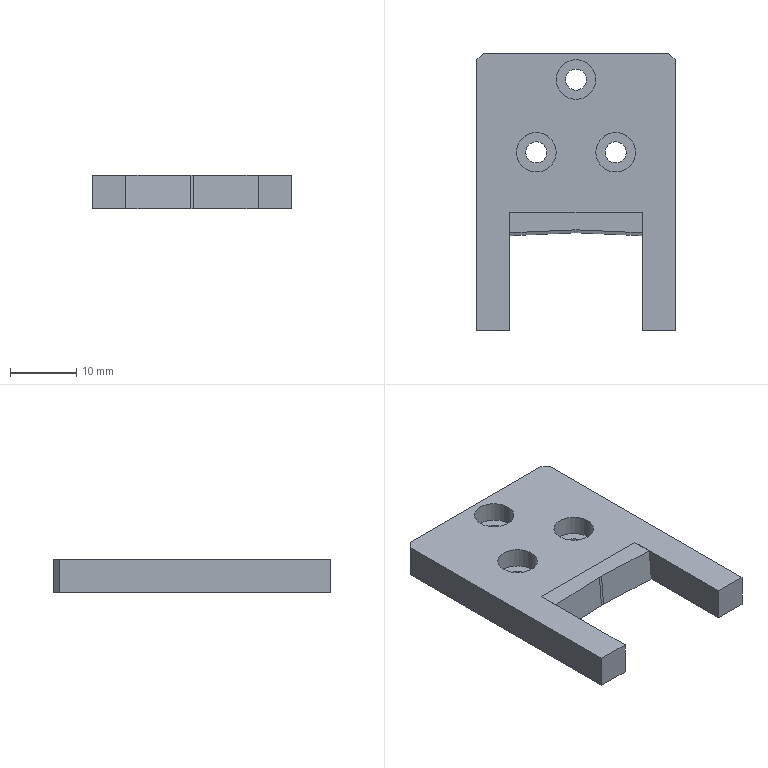Part | SolidWorks | features ICE 3, Chamfer 2, Extrusion 1, Fillet 1, HoleWzd 1 | 2 solids | 35 faces | box 30 x 42 x 5 mm | volume 4509 mm3 | plane 22 | cylinder 13 | commonest cylinder face diameters 3.2 x6 6 x6 10 x1
STEP:
#1=CARTESIAN_POINT('',(-18.,-4.,-0.5));
#2=VERTEX_POINT('',#1);
#3=CARTESIAN_POINT('',(-12.,-4.,-0.5));
#4=VERTEX_POINT('',#3);
#5=CARTESIAN_POINT('',(-15.,-4.,-0.5));
#6=DIRECTION('',(0.,0.,1.));
#7=DIRECTION('',(1.,0.,0.));
#8=AXIS2_PLACEMENT_3D('',#5,#6,#7);
#9=CIRCLE('',#8,3.);
#10=EDGE_CURVE('',#2,#4,#9,.T.);
#11=ORIENTED_EDGE('',*,*,#10,.F.);
#12=CARTESIAN_POINT('',(-18.,-4.,2.5));
#13=VERTEX_POINT('',#12);
#14=CARTESIAN_POINT('',(-18.,-4.,2.5));
#15=DIRECTION('',(0.,0.,1.));
#16=VECTOR('',#15,1000.);
#17=LINE('',#14,#16);
#18=EDGE_CURVE('',#2,#13,#17,.T.);
#19=ORIENTED_EDGE('',*,*,#18,.T.);
#20=CARTESIAN_POINT('',(-12.,-4.,2.5));
#21=VERTEX_POINT('',#20);
#22=CARTESIAN_POINT('',(-15.,-4.,2.5));
#23=DIRECTION('',(0.,0.,1.));
#24=DIRECTION('',(1.,0.,0.));
#25=AXIS2_PLACEMENT_3D('',#22,#23,#24);
#26=CIRCLE('',#25,3.);
#27=EDGE_CURVE('',#13,#21,#26,.T.);
#28=ORIENTED_EDGE('',*,*,#27,.T.);
#29=CARTESIAN_POINT('',(-12.,-4.,2.5));
#30=DIRECTION('',(0.,0.,1.));
#31=VECTOR('',#30,1000.);
#32=LINE('',#29,#31);
#33=EDGE_CURVE('',#4,#21,#32,.T.);
#34=ORIENTED_EDGE('',*,*,#33,.F.);
#35=EDGE_LOOP('',(#11,#19,#28,#34));
#36=FACE_OUTER_BOUND('',#35,.T.);
#37=CARTESIAN_POINT('',(-15.,-4.,2.5));
#38=DIRECTION('',(0.,0.,1.));
#39=DIRECTION('',(1.,0.,0.));
#40=AXIS2_PLACEMENT_3D('',#37,#38,#39);
#41=CYLINDRICAL_SURFACE('',#40,3.);
#42=ADVANCED_FACE('',(#36),#41,.F.);
#43=CARTESIAN_POINT('',(-16.6,-4.,-2.5));
#44=VERTEX_POINT('',#43);
#45=CARTESIAN_POINT('',(-13.4,-4.,-2.5));
#46=VERTEX_POINT('',#45);
#47=CARTESIAN_POINT('',(-15.,-4.,-2.5));
#48=DIRECTION('',(0.,0.,1.));
#49=DIRECTION('',(1.,0.,0.));
#50=AXIS2_PLACEMENT_3D('',#47,#48,#49);
#51=CIRCLE('',#50,1.6);
#52=EDGE_CURVE('',#44,#46,#51,.T.);
#53=ORIENTED_EDGE('',*,*,#52,.F.);
#54=CARTESIAN_POINT('',(-16.6,-4.,-0.5));
#55=VERTEX_POINT('',#54);
#56=CARTESIAN_POINT('',(-16.6,-4.,2.5));
#57=DIRECTION('',(0.,0.,1.));
#58=VECTOR('',#57,1000.);
#59=LINE('',#56,#58);
#60=EDGE_CURVE('',#44,#55,#59,.T.);
#61=ORIENTED_EDGE('',*,*,#60,.T.);
#62=CARTESIAN_POINT('',(-13.4,-4.,-0.5));
#63=VERTEX_POINT('',#62);
#64=CARTESIAN_POINT('',(-15.,-4.,-0.5));
#65=DIRECTION('',(0.,0.,1.));
#66=DIRECTION('',(1.,0.,0.));
#67=AXIS2_PLACEMENT_3D('',#64,#65,#66);
#68=CIRCLE('',#67,1.6);
#69=EDGE_CURVE('',#55,#63,#68,.T.);
#70=ORIENTED_EDGE('',*,*,#69,.T.);
#71=CARTESIAN_POINT('',(-13.4,-4.,2.5));
#72=DIRECTION('',(0.,0.,1.));
#73=VECTOR('',#72,1000.);
#74=LINE('',#71,#73);
#75=EDGE_CURVE('',#46,#63,#74,.T.);
#76=ORIENTED_EDGE('',*,*,#75,.F.);
#77=EDGE_LOOP('',(#53,#61,#70,#76));
#78=FACE_OUTER_BOUND('',#77,.T.);
#79=CARTESIAN_POINT('',(-15.,-4.,2.5));
#80=DIRECTION('',(0.,0.,1.));
#81=DIRECTION('',(1.,0.,0.));
#82=AXIS2_PLACEMENT_3D('',#79,#80,#81);
#83=CYLINDRICAL_SURFACE('',#82,1.6);
#84=ADVANCED_FACE('',(#78),#83,.F.);
#85=CARTESIAN_POINT('',(-24.,-15.,-0.5));
#86=VERTEX_POINT('',#85);
#87=CARTESIAN_POINT('',(-18.,-15.,-0.5));
#88=VERTEX_POINT('',#87);
#89=CARTESIAN_POINT('',(-21.,-15.,-0.5));
#90=DIRECTION('',(0.,0.,1.));
#91=DIRECTION('',(1.,0.,0.));
#92=AXIS2_PLACEMENT_3D('',#89,#90,#91);
#93=CIRCLE('',#92,3.);
#94=EDGE_CURVE('',#86,#88,#93,.T.);
#95=ORIENTED_EDGE('',*,*,#94,.F.);
#96=CARTESIAN_POINT('',(-24.,-15.,2.5));
#97=VERTEX_POINT('',#96);
#98=CARTESIAN_POINT('',(-24.,-15.,2.5));
#99=DIRECTION('',(0.,0.,1.));
#100=VECTOR('',#99,1000.);
#101=LINE('',#98,#100);
#102=EDGE_CURVE('',#86,#97,#101,.T.);
#103=ORIENTED_EDGE('',*,*,#102,.T.);
#104=CARTESIAN_POINT('',(-18.,-15.,2.5));
#105=VERTEX_POINT('',#104);
#106=CARTESIAN_POINT('',(-21.,-15.,2.5));
#107=DIRECTION('',(0.,0.,1.));
#108=DIRECTION('',(1.,0.,0.));
#109=AXIS2_PLACEMENT_3D('',#106,#107,#108);
#110=CIRCLE('',#109,3.);
#111=EDGE_CURVE('',#97,#105,#110,.T.);
#112=ORIENTED_EDGE('',*,*,#111,.T.);
#113=CARTESIAN_POINT('',(-18.,-15.,2.5));
#114=DIRECTION('',(0.,0.,1.));
#115=VECTOR('',#114,1000.);
#116=LINE('',#113,#115);
#117=EDGE_CURVE('',#88,#105,#116,.T.);
#118=ORIENTED_EDGE('',*,*,#117,.F.);
#119=EDGE_LOOP('',(#95,#103,#112,#118));
#120=FACE_OUTER_BOUND('',#119,.T.);
#121=CARTESIAN_POINT('',(-21.,-15.,2.5));
#122=DIRECTION('',(0.,0.,1.));
#123=DIRECTION('',(1.,0.,0.));
#124=AXIS2_PLACEMENT_3D('',#121,#122,#123);
#125=CYLINDRICAL_SURFACE('',#124,3.);
#126=ADVANCED_FACE('',(#120),#125,.F.);
#127=CARTESIAN_POINT('',(-22.6,-15.,-2.5));
#128=VERTEX_POINT('',#127);
#129=CARTESIAN_POINT('',(-19.4,-15.,-2.5));
#130=VERTEX_POINT('',#129);
#131=CARTESIAN_POINT('',(-21.,-15.,-2.5));
#132=DIRECTION('',(0.,0.,1.));
#133=DIRECTION('',(1.,0.,0.));
#134=AXIS2_PLACEMENT_3D('',#131,#132,#133);
#135=CIRCLE('',#134,1.6);
#136=EDGE_CURVE('',#128,#130,#135,.T.);
#137=ORIENTED_EDGE('',*,*,#136,.F.);
#138=CARTESIAN_POINT('',(-22.6,-15.,-0.5));
#139=VERTEX_POINT('',#138);
#140=CARTESIAN_POINT('',(-22.6,-15.,2.5));
#141=DIRECTION('',(0.,0.,1.));
#142=VECTOR('',#141,1000.);
#143=LINE('',#140,#142);
#144=EDGE_CURVE('',#128,#139,#143,.T.);
#145=ORIENTED_EDGE('',*,*,#144,.T.);
#146=CARTESIAN_POINT('',(-19.4,-15.,-0.5));
#147=VERTEX_POINT('',#146);
#148=CARTESIAN_POINT('',(-21.,-15.,-0.5));
#149=DIRECTION('',(0.,0.,1.));
#150=DIRECTION('',(1.,0.,0.));
#151=AXIS2_PLACEMENT_3D('',#148,#149,#150);
#152=CIRCLE('',#151,1.6);
#153=EDGE_CURVE('',#139,#147,#152,.T.);
#154=ORIENTED_EDGE('',*,*,#153,.T.);
#155=CARTESIAN_POINT('',(-19.4,-15.,2.5));
#156=DIRECTION('',(0.,0.,1.));
#157=VECTOR('',#156,1000.);
#158=LINE('',#155,#157);
#159=EDGE_CURVE('',#130,#147,#158,.T.);
#160=ORIENTED_EDGE('',*,*,#159,.F.);
#161=EDGE_LOOP('',(#137,#145,#154,#160));
#162=FACE_OUTER_BOUND('',#161,.T.);
#163=CARTESIAN_POINT('',(-21.,-15.,2.5));
#164=DIRECTION('',(0.,0.,1.));
#165=DIRECTION('',(1.,0.,0.));
#166=AXIS2_PLACEMENT_3D('',#163,#164,#165);
#167=CYLINDRICAL_SURFACE('',#166,1.6);
#168=ADVANCED_FACE('',(#162),#167,.F.);
#169=CARTESIAN_POINT('',(-12.,-15.,-0.5));
#170=VERTEX_POINT('',#169);
#171=CARTESIAN_POINT('',(-6.,-15.,-0.5));
#172=VERTEX_POINT('',#171);
#173=CARTESIAN_POINT('',(-9.,-15.,-0.5));
#174=DIRECTION('',(0.,0.,1.));
#175=DIRECTION('',(1.,0.,0.));
#176=AXIS2_PLACEMENT_3D('',#173,#174,#175);
#177=CIRCLE('',#176,3.);
#178=EDGE_CURVE('',#170,#172,#177,.T.);
#179=ORIENTED_EDGE('',*,*,#178,.F.);
#180=CARTESIAN_POINT('',(-12.,-15.,2.5));
#181=VERTEX_POINT('',#180);
#182=CARTESIAN_POINT('',(-12.,-15.,2.5));
#183=DIRECTION('',(0.,0.,1.));
#184=VECTOR('',#183,1000.);
#185=LINE('',#182,#184);
#186=EDGE_CURVE('',#170,#181,#185,.T.);
#187=ORIENTED_EDGE('',*,*,#186,.T.);
#188=CARTESIAN_POINT('',(-6.,-15.,2.5));
#189=VERTEX_POINT('',#188);
#190=CARTESIAN_POINT('',(-9.,-15.,2.5));
#191=DIRECTION('',(0.,0.,1.));
#192=DIRECTION('',(1.,0.,0.));
#193=AXIS2_PLACEMENT_3D('',#190,#191,#192);
#194=CIRCLE('',#193,3.);
#195=EDGE_CURVE('',#181,#189,#194,.T.);
#196=ORIENTED_EDGE('',*,*,#195,.T.);
#197=CARTESIAN_POINT('',(-6.,-15.,2.5));
#198=DIRECTION('',(0.,0.,1.));
#199=VECTOR('',#198,1000.);
#200=LINE('',#197,#199);
#201=EDGE_CURVE('',#172,#189,#200,.T.);
#202=ORIENTED_EDGE('',*,*,#201,.F.);
#203=EDGE_LOOP('',(#179,#187,#196,#202));
#204=FACE_OUTER_BOUND('',#203,.T.);
#205=CARTESIAN_POINT('',(-9.,-15.,2.5));
#206=DIRECTION('',(0.,0.,1.));
#207=DIRECTION('',(1.,0.,0.));
#208=AXIS2_PLACEMENT_3D('',#205,#206,#207);
#209=CYLINDRICAL_SURFACE('',#208,3.);
#210=ADVANCED_FACE('',(#204),#209,.F.);
#211=CARTESIAN_POINT('',(-10.6,-15.,-2.5));
#212=VERTEX_POINT('',#211);
#213=CARTESIAN_POINT('',(-7.4,-15.,-2.5));
#214=VERTEX_POINT('',#213);
#215=CARTESIAN_POINT('',(-9.,-15.,-2.5));
#216=DIRECTION('',(0.,0.,1.));
#217=DIRECTION('',(1.,0.,0.));
#218=AXIS2_PLACEMENT_3D('',#215,#216,#217);
#219=CIRCLE('',#218,1.6);
#220=EDGE_CURVE('',#212,#214,#219,.T.);
#221=ORIENTED_EDGE('',*,*,#220,.F.);
#222=CARTESIAN_POINT('',(-10.6,-15.,-0.5));
#223=VERTEX_POINT('',#222);
#224=CARTESIAN_POINT('',(-10.6,-15.,2.5));
#225=DIRECTION('',(0.,0.,1.));
#226=VECTOR('',#225,1000.);
#227=LINE('',#224,#226);
#228=EDGE_CURVE('',#212,#223,#227,.T.);
#229=ORIENTED_EDGE('',*,*,#228,.T.);
#230=CARTESIAN_POINT('',(-7.4,-15.,-0.5));
#231=VERTEX_POINT('',#230);
#232=CARTESIAN_POINT('',(-9.,-15.,-0.5));
#233=DIRECTION('',(0.,0.,1.));
#234=DIRECTION('',(1.,0.,0.));
#235=AXIS2_PLACEMENT_3D('',#232,#233,#234);
#236=CIRCLE('',#235,1.6);
#237=EDGE_CURVE('',#223,#231,#236,.T.);
#238=ORIENTED_EDGE('',*,*,#237,.T.);
#239=CARTESIAN_POINT('',(-7.4,-15.,2.5));
#240=DIRECTION('',(0.,0.,1.));
#241=VECTOR('',#240,1000.);
#242=LINE('',#239,#241);
#243=EDGE_CURVE('',#214,#231,#242,.T.);
#244=ORIENTED_EDGE('',*,*,#243,.F.);
#245=EDGE_LOOP('',(#221,#229,#238,#244));
#246=FACE_OUTER_BOUND('',#245,.T.);
#247=CARTESIAN_POINT('',(-9.,-15.,2.5));
#248=DIRECTION('',(0.,0.,1.));
#249=DIRECTION('',(1.,0.,0.));
#250=AXIS2_PLACEMENT_3D('',#247,#248,#249);
#251=CYLINDRICAL_SURFACE('',#250,1.6);
#252=ADVANCED_FACE('',(#246),#251,.F.);
#253=CARTESIAN_POINT('',(0.,-42.,-2.5));
#254=VERTEX_POINT('',#253);
#255=CARTESIAN_POINT('',(0.,-1.,-2.5));
#256=VERTEX_POINT('',#255);
#257=CARTESIAN_POINT('',(0.,0.,-2.5));
#258=DIRECTION('',(0.,1.,0.));
#259=VECTOR('',#258,1000.);
#260=LINE('',#257,#259);
#261=EDGE_CURVE('',#254,#256,#260,.T.);
#262=ORIENTED_EDGE('',*,*,#261,.T.);
#263=CARTESIAN_POINT('',(0.,-1.,2.5));
#264=VERTEX_POINT('',#263);
#265=CARTESIAN_POINT('',(0.,-1.,2.5));
#266=DIRECTION('',(0.,0.,1.));
#267=VECTOR('',#266,1000.);
#268=LINE('',#265,#267);
#269=EDGE_CURVE('',#256,#264,#268,.T.);
#270=ORIENTED_EDGE('',*,*,#269,.T.);
#271=CARTESIAN_POINT('',(0.,-42.,2.5));
#272=VERTEX_POINT('',#271);
#273=CARTESIAN_POINT('',(0.,0.,2.5));
#274=DIRECTION('',(0.,1.,0.));
#275=VECTOR('',#274,1000.);
#276=LINE('',#273,#275);
#277=EDGE_CURVE('',#272,#264,#276,.T.);
#278=ORIENTED_EDGE('',*,*,#277,.F.);
#279=CARTESIAN_POINT('',(0.,-42.,2.5));
#280=DIRECTION('',(0.,0.,-1.));
#281=VECTOR('',#280,1000.);
#282=LINE('',#279,#281);
#283=EDGE_CURVE('',#272,#254,#282,.T.);
#284=ORIENTED_EDGE('',*,*,#283,.T.);
#285=EDGE_LOOP('',(#262,#270,#278,#284));
#286=FACE_OUTER_BOUND('',#285,.T.);
#287=CARTESIAN_POINT('',(0.,0.,2.5));
#288=DIRECTION('',(-1.,0.,0.));
#289=DIRECTION('',(0.,-1.,0.));
#290=AXIS2_PLACEMENT_3D('',#287,#288,#289);
#291=PLANE('',#290);
#292=ADVANCED_FACE('',(#286),#291,.F.);
#293=CARTESIAN_POINT('',(-1.,0.,2.5));
#294=VERTEX_POINT('',#293);
#295=CARTESIAN_POINT('',(-29.,0.,2.5));
#296=VERTEX_POINT('',#295);
#297=CARTESIAN_POINT('',(0.,0.,2.5));
#298=DIRECTION('',(-1.,0.,0.));
#299=VECTOR('',#298,1000.);
#300=LINE('',#297,#299);
#301=EDGE_CURVE('',#294,#296,#300,.T.);
#302=ORIENTED_EDGE('',*,*,#301,.F.);
#303=CARTESIAN_POINT('',(-1.,0.,-2.5));
#304=VERTEX_POINT('',#303);
#305=CARTESIAN_POINT('',(-1.,0.,2.5));
#306=DIRECTION('',(0.,0.,-1.));
#307=VECTOR('',#306,1000.);
#308=LINE('',#305,#307);
#309=EDGE_CURVE('',#294,#304,#308,.T.);
#310=ORIENTED_EDGE('',*,*,#309,.T.);
#311=CARTESIAN_POINT('',(-29.,0.,-2.5));
#312=VERTEX_POINT('',#311);
#313=CARTESIAN_POINT('',(0.,0.,-2.5));
#314=DIRECTION('',(-1.,0.,0.));
#315=VECTOR('',#314,1000.);
#316=LINE('',#313,#315);
#317=EDGE_CURVE('',#304,#312,#316,.T.);
#318=ORIENTED_EDGE('',*,*,#317,.T.);
#319=CARTESIAN_POINT('',(-29.,0.,2.5));
#320=DIRECTION('',(0.,0.,1.));
#321=VECTOR('',#320,1000.);
#322=LINE('',#319,#321);
#323=EDGE_CURVE('',#312,#296,#322,.T.);
#324=ORIENTED_EDGE('',*,*,#323,.T.);
#325=EDGE_LOOP('',(#302,#310,#318,#324));
#326=FACE_OUTER_BOUND('',#325,.T.);
#327=CARTESIAN_POINT('',(0.,0.,2.5));
#328=DIRECTION('',(0.,-1.,0.));
#329=DIRECTION('',(1.,0.,0.));
#330=AXIS2_PLACEMENT_3D('',#327,#328,#329);
#331=PLANE('',#330);
#332=ADVANCED_FACE('',(#326),#331,.F.);
#333=CARTESIAN_POINT('',(-30.,-1.,2.5));
#334=VERTEX_POINT('',#333);
#335=CARTESIAN_POINT('',(-30.,-42.,2.5));
#336=VERTEX_POINT('',#335);
#337=CARTESIAN_POINT('',(-30.,0.,2.5));
#338=DIRECTION('',(0.,-1.,0.));
#339=VECTOR('',#338,1000.);
#340=LINE('',#337,#339);
#341=EDGE_CURVE('',#334,#336,#340,.T.);
#342=ORIENTED_EDGE('',*,*,#341,.F.);
#343=CARTESIAN_POINT('',(-30.,-1.,-2.5));
#344=VERTEX_POINT('',#343);
#345=CARTESIAN_POINT('',(-30.,-1.,2.5));
#346=DIRECTION('',(0.,0.,-1.));
#347=VECTOR('',#346,1000.);
#348=LINE('',#345,#347);
#349=EDGE_CURVE('',#334,#344,#348,.T.);
#350=ORIENTED_EDGE('',*,*,#349,.T.);
#351=CARTESIAN_POINT('',(-30.,-42.,-2.5));
#352=VERTEX_POINT('',#351);
#353=CARTESIAN_POINT('',(-30.,0.,-2.5));
#354=DIRECTION('',(0.,-1.,0.));
#355=VECTOR('',#354,1000.);
#356=LINE('',#353,#355);
#357=EDGE_CURVE('',#344,#352,#356,.T.);
#358=ORIENTED_EDGE('',*,*,#357,.T.);
#359=CARTESIAN_POINT('',(-30.,-42.,2.5));
#360=DIRECTION('',(0.,0.,-1.));
#361=VECTOR('',#360,1000.);
#362=LINE('',#359,#361);
#363=EDGE_CURVE('',#336,#352,#362,.T.);
#364=ORIENTED_EDGE('',*,*,#363,.F.);
#365=EDGE_LOOP('',(#342,#350,#358,#364));
#366=FACE_OUTER_BOUND('',#365,.T.);
#367=CARTESIAN_POINT('',(-30.,0.,2.5));
#368=DIRECTION('',(1.,0.,0.));
#369=DIRECTION('',(0.,1.,0.));
#370=AXIS2_PLACEMENT_3D('',#367,#368,#369);
#371=PLANE('',#370);
#372=ADVANCED_FACE('',(#366),#371,.F.);
#373=CARTESIAN_POINT('',(-25.,-42.,-2.5));
#374=VERTEX_POINT('',#373);
#375=CARTESIAN_POINT('',(-25.,-42.,-2.5));
#376=DIRECTION('',(1.,0.,0.));
#377=VECTOR('',#376,1000.);
#378=LINE('',#375,#377);
#379=EDGE_CURVE('',#352,#374,#378,.T.);
#380=ORIENTED_EDGE('',*,*,#379,.T.);
#381=CARTESIAN_POINT('',(-25.,-42.,2.5));
#382=VERTEX_POINT('',#381);
#383=CARTESIAN_POINT('',(-25.,-42.,2.5));
#384=DIRECTION('',(0.,0.,-1.));
#385=VECTOR('',#384,1000.);
#386=LINE('',#383,#385);
#387=EDGE_CURVE('',#382,#374,#386,.T.);
#388=ORIENTED_EDGE('',*,*,#387,.F.);
#389=CARTESIAN_POINT('',(-25.,-42.,2.5));
#390=DIRECTION('',(1.,0.,0.));
#391=VECTOR('',#390,1000.);
#392=LINE('',#389,#391);
#393=EDGE_CURVE('',#336,#382,#392,.T.);
#394=ORIENTED_EDGE('',*,*,#393,.F.);
#395=ORIENTED_EDGE('',*,*,#363,.T.);
#396=EDGE_LOOP('',(#380,#388,#394,#395));
#397=FACE_OUTER_BOUND('',#396,.T.);
#398=CARTESIAN_POINT('',(-25.,-42.,2.5));
#399=DIRECTION('',(0.,1.,0.));
#400=DIRECTION('',(-1.,0.,0.));
#401=AXIS2_PLACEMENT_3D('',#398,#399,#400);
#402=PLANE('',#401);
#403=ADVANCED_FACE('',(#397),#402,.F.);
#404=CARTESIAN_POINT('',(-25.,-24.1,-2.5));
#405=VERTEX_POINT('',#404);
#406=CARTESIAN_POINT('',(-25.,-24.1,-2.5));
#407=DIRECTION('',(0.,1.,0.));
#408=VECTOR('',#407,1000.);
#409=LINE('',#406,#408);
#410=EDGE_CURVE('',#374,#405,#409,.T.);
#411=ORIENTED_EDGE('',*,*,#410,.T.);
#412=CARTESIAN_POINT('',(-25.,-24.1,2.5));
#413=VERTEX_POINT('',#412);
#414=CARTESIAN_POINT('',(-25.,-24.1,2.5));
#415=DIRECTION('',(0.,0.,-1.));
#416=VECTOR('',#415,1000.);
#417=LINE('',#414,#416);
#418=EDGE_CURVE('',#413,#405,#417,.T.);
#419=ORIENTED_EDGE('',*,*,#418,.F.);
#420=CARTESIAN_POINT('',(-25.,-24.1,2.5));
#421=DIRECTION('',(0.,1.,0.));
#422=VECTOR('',#421,1000.);
#423=LINE('',#420,#422);
#424=EDGE_CURVE('',#382,#413,#423,.T.);
#425=ORIENTED_EDGE('',*,*,#424,.F.);
#426=ORIENTED_EDGE('',*,*,#387,.T.);
#427=EDGE_LOOP('',(#411,#419,#425,#426));
#428=FACE_OUTER_BOUND('',#427,.T.);
#429=CARTESIAN_POINT('',(-25.,-24.1,2.5));
#430=DIRECTION('',(-1.,0.,0.));
#431=DIRECTION('',(0.,0.,1.));
#432=AXIS2_PLACEMENT_3D('',#429,#430,#431);
#433=PLANE('',#432);
#434=ADVANCED_FACE('',(#428),#433,.F.);
#435=CARTESIAN_POINT('',(-5.,-24.1,-2.5));
#436=VERTEX_POINT('',#435);
#437=CARTESIAN_POINT('',(-25.,-24.1,-2.5));
#438=DIRECTION('',(1.,0.,0.));
#439=VECTOR('',#438,1000.);
#440=LINE('',#437,#439);
#441=EDGE_CURVE('',#405,#436,#440,.T.);
#442=ORIENTED_EDGE('',*,*,#441,.T.);
#443=CARTESIAN_POINT('',(-5.,-24.1,2.5));
#444=VERTEX_POINT('',#443);
#445=CARTESIAN_POINT('',(-5.,-24.1,2.5));
#446=DIRECTION('',(0.,0.,-1.));
#447=VECTOR('',#446,1000.);
#448=LINE('',#445,#447);
#449=EDGE_CURVE('',#444,#436,#448,.T.);
#450=ORIENTED_EDGE('',*,*,#449,.F.);
#451=CARTESIAN_POINT('',(-25.,-24.1,2.5));
#452=DIRECTION('',(1.,0.,0.));
#453=VECTOR('',#452,1000.);
#454=LINE('',#451,#453);
#455=EDGE_CURVE('',#413,#444,#454,.T.);
#456=ORIENTED_EDGE('',*,*,#455,.F.);
#457=ORIENTED_EDGE('',*,*,#418,.T.);
#458=EDGE_LOOP('',(#442,#450,#456,#457));
#459=FACE_OUTER_BOUND('',#458,.T.);
#460=CARTESIAN_POINT('',(-25.,-24.1,2.5));
#461=DIRECTION('',(0.,1.,0.));
#462=DIRECTION('',(0.,0.,1.));
#463=AXIS2_PLACEMENT_3D('',#460,#461,#462);
#464=PLANE('',#463);
#465=ADVANCED_FACE('',(#459),#464,.F.);
#466=CARTESIAN_POINT('',(-5.,-42.,-2.5));
#467=VERTEX_POINT('',#466);
#468=CARTESIAN_POINT('',(-5.,-42.,-2.5));
#469=DIRECTION('',(0.,-1.,0.));
#470=VECTOR('',#469,1000.);
#471=LINE('',#468,#470);
#472=EDGE_CURVE('',#436,#467,#471,.T.);
#473=ORIENTED_EDGE('',*,*,#472,.T.);
#474=CARTESIAN_POINT('',(-5.,-42.,2.5));
#475=VERTEX_POINT('',#474);
#476=CARTESIAN_POINT('',(-5.,-42.,2.5));
#477=DIRECTION('',(0.,0.,-1.));
#478=VECTOR('',#477,1000.);
#479=LINE('',#476,#478);
#480=EDGE_CURVE('',#475,#467,#479,.T.);
#481=ORIENTED_EDGE('',*,*,#480,.F.);
#482=CARTESIAN_POINT('',(-5.,-42.,2.5));
#483=DIRECTION('',(0.,-1.,0.));
#484=VECTOR('',#483,1000.);
#485=LINE('',#482,#484);
#486=EDGE_CURVE('',#444,#475,#485,.T.);
#487=ORIENTED_EDGE('',*,*,#486,.F.);
#488=ORIENTED_EDGE('',*,*,#449,.T.);
#489=EDGE_LOOP('',(#473,#481,#487,#488));
#490=FACE_OUTER_BOUND('',#489,.T.);
#491=CARTESIAN_POINT('',(-5.,-42.,2.5));
#492=DIRECTION('',(1.,0.,0.));
#493=DIRECTION('',(0.,1.,0.));
#494=AXIS2_PLACEMENT_3D('',#491,#492,#493);
#495=PLANE('',#494);
#496=ADVANCED_FACE('',(#490),#495,.F.);
#497=CARTESIAN_POINT('',(0.,-42.,-2.5));
#498=DIRECTION('',(1.,0.,0.));
#499=VECTOR('',#498,1000.);
#500=LINE('',#497,#499);
#501=EDGE_CURVE('',#467,#254,#500,.T.);
#502=ORIENTED_EDGE('',*,*,#501,.T.);
#503=ORIENTED_EDGE('',*,*,#283,.F.);
#504=CARTESIAN_POINT('',(0.,-42.,2.5));
#505=DIRECTION('',(1.,0.,0.));
#506=VECTOR('',#505,1000.);
#507=LINE('',#504,#506);
#508=EDGE_CURVE('',#475,#272,#507,.T.);
#509=ORIENTED_EDGE('',*,*,#508,.F.);
#510=ORIENTED_EDGE('',*,*,#480,.T.);
#511=EDGE_LOOP('',(#502,#503,#509,#510));
#512=FACE_OUTER_BOUND('',#511,.T.);
#513=CARTESIAN_POINT('',(0.,-42.,2.5));
#514=DIRECTION('',(0.,1.,0.));
#515=DIRECTION('',(0.,0.,1.));
#516=AXIS2_PLACEMENT_3D('',#513,#514,#515);
#517=PLANE('',#516);
#518=ADVANCED_FACE('',(#512),#517,.F.);
#519=CARTESIAN_POINT('',(-15.,-4.,2.5));
#520=DIRECTION('',(0.,0.,1.));
#521=DIRECTION('',(1.,0.,0.));
#522=AXIS2_PLACEMENT_3D('',#519,#520,#521);
#523=CIRCLE('',#522,3.);
#524=EDGE_CURVE('',#21,#13,#523,.T.);
#525=ORIENTED_EDGE('',*,*,#524,.F.);
#526=ORIENTED_EDGE('',*,*,#27,.F.);
#527=EDGE_LOOP('',(#525,#526));
#528=FACE_BOUND('',#527,.T.);
#529=CARTESIAN_POINT('',(-21.,-15.,2.5));
#530=DIRECTION('',(0.,0.,1.));
#531=DIRECTION('',(1.,0.,0.));
#532=AXIS2_PLACEMENT_3D('',#529,#530,#531);
#533=CIRCLE('',#532,3.);
#534=EDGE_CURVE('',#105,#97,#533,.T.);
#535=ORIENTED_EDGE('',*,*,#534,.F.);
#536=ORIENTED_EDGE('',*,*,#111,.F.);
#537=EDGE_LOOP('',(#535,#536));
#538=FACE_BOUND('',#537,.T.);
#539=CARTESIAN_POINT('',(-9.,-15.,2.5));
#540=DIRECTION('',(0.,0.,1.));
#541=DIRECTION('',(1.,0.,0.));
#542=AXIS2_PLACEMENT_3D('',#539,#540,#541);
#543=CIRCLE('',#542,3.);
#544=EDGE_CURVE('',#189,#181,#543,.T.);
#545=ORIENTED_EDGE('',*,*,#544,.F.);
#546=ORIENTED_EDGE('',*,*,#195,.F.);
#547=EDGE_LOOP('',(#545,#546));
#548=FACE_BOUND('',#547,.T.);
#549=ORIENTED_EDGE('',*,*,#277,.T.);
#550=CARTESIAN_POINT('',(-1.,0.,2.5));
#551=DIRECTION('',(-0.7071,0.7071,0.));
#552=VECTOR('',#551,1000.);
#553=LINE('',#550,#552);
#554=EDGE_CURVE('',#264,#294,#553,.T.);
#555=ORIENTED_EDGE('',*,*,#554,.T.);
#556=ORIENTED_EDGE('',*,*,#301,.T.);
#557=CARTESIAN_POINT('',(-30.,-1.,2.5));
#558=DIRECTION('',(-0.7071,-0.7071,0.));
#559=VECTOR('',#558,1000.);
#560=LINE('',#557,#559);
#561=EDGE_CURVE('',#296,#334,#560,.T.);
#562=ORIENTED_EDGE('',*,*,#561,.T.);
#563=ORIENTED_EDGE('',*,*,#341,.T.);
#564=ORIENTED_EDGE('',*,*,#393,.T.);
#565=ORIENTED_EDGE('',*,*,#424,.T.);
#566=ORIENTED_EDGE('',*,*,#455,.T.);
#567=ORIENTED_EDGE('',*,*,#486,.T.);
#568=ORIENTED_EDGE('',*,*,#508,.T.);
#569=EDGE_LOOP('',(#549,#555,#556,#562,#563,#564,#565,#566,#567,#568));
#570=FACE_OUTER_BOUND('',#569,.T.);
#571=CARTESIAN_POINT('',(0.,-42.,2.5));
#572=DIRECTION('',(0.,0.,-1.));
#573=DIRECTION('',(-1.,0.,0.));
#574=AXIS2_PLACEMENT_3D('',#571,#572,#573);
#575=PLANE('',#574);
#576=ADVANCED_FACE('',(#528,#538,#548,#570),#575,.F.);
#577=CARTESIAN_POINT('',(-15.,-4.,-2.5));
#578=DIRECTION('',(0.,0.,1.));
#579=DIRECTION('',(1.,0.,0.));
#580=AXIS2_PLACEMENT_3D('',#577,#578,#579);
#581=CIRCLE('',#580,1.6);
#582=EDGE_CURVE('',#46,#44,#581,.T.);
#583=ORIENTED_EDGE('',*,*,#582,.T.);
#584=ORIENTED_EDGE('',*,*,#52,.T.);
#585=EDGE_LOOP('',(#583,#584));
#586=FACE_BOUND('',#585,.T.);
#587=CARTESIAN_POINT('',(-21.,-15.,-2.5));
#588=DIRECTION('',(0.,0.,1.));
#589=DIRECTION('',(1.,0.,0.));
#590=AXIS2_PLACEMENT_3D('',#587,#588,#589);
#591=CIRCLE('',#590,1.6);
#592=EDGE_CURVE('',#130,#128,#591,.T.);
#593=ORIENTED_EDGE('',*,*,#592,.T.);
#594=ORIENTED_EDGE('',*,*,#136,.T.);
#595=EDGE_LOOP('',(#593,#594));
#596=FACE_BOUND('',#595,.T.);
#597=CARTESIAN_POINT('',(-9.,-15.,-2.5));
#598=DIRECTION('',(0.,0.,1.));
#599=DIRECTION('',(1.,0.,0.));
#600=AXIS2_PLACEMENT_3D('',#597,#598,#599);
#601=CIRCLE('',#600,1.6);
#602=EDGE_CURVE('',#214,#212,#601,.T.);
#603=ORIENTED_EDGE('',*,*,#602,.T.);
#604=ORIENTED_EDGE('',*,*,#220,.T.);
#605=EDGE_LOOP('',(#603,#604));
#606=FACE_BOUND('',#605,.T.);
#607=ORIENTED_EDGE('',*,*,#317,.F.);
#608=CARTESIAN_POINT('',(20.5,-21.5,-2.5));
#609=DIRECTION('',(0.7071,-0.7071,0.));
#610=VECTOR('',#609,1000.);
#611=LINE('',#608,#610);
#612=EDGE_CURVE('',#304,#256,#611,.T.);
#613=ORIENTED_EDGE('',*,*,#612,.T.);
#614=ORIENTED_EDGE('',*,*,#261,.F.);
#615=ORIENTED_EDGE('',*,*,#501,.F.);
#616=ORIENTED_EDGE('',*,*,#472,.F.);
#617=ORIENTED_EDGE('',*,*,#441,.F.);
#618=ORIENTED_EDGE('',*,*,#410,.F.);
#619=ORIENTED_EDGE('',*,*,#379,.F.);
#620=ORIENTED_EDGE('',*,*,#357,.F.);
#621=CARTESIAN_POINT('',(-35.5,-6.5,-2.5));
#622=DIRECTION('',(0.7071,0.7071,0.));
#623=VECTOR('',#622,1000.);
#624=LINE('',#621,#623);
#625=EDGE_CURVE('',#344,#312,#624,.T.);
#626=ORIENTED_EDGE('',*,*,#625,.T.);
#627=EDGE_LOOP('',(#607,#613,#614,#615,#616,#617,#618,#619,#620,#626));
#628=FACE_OUTER_BOUND('',#627,.T.);
#629=CARTESIAN_POINT('',(0.,-42.,-2.5));
#630=DIRECTION('',(0.,0.,-1.));
#631=DIRECTION('',(-1.,0.,0.));
#632=AXIS2_PLACEMENT_3D('',#629,#630,#631);
#633=PLANE('',#632);
#634=ADVANCED_FACE('',(#586,#596,#606,#628),#633,.T.);
#635=ORIENTED_EDGE('',*,*,#228,.F.);
#636=ORIENTED_EDGE('',*,*,#602,.F.);
#637=ORIENTED_EDGE('',*,*,#243,.T.);
#638=CARTESIAN_POINT('',(-9.,-15.,-0.5));
#639=DIRECTION('',(0.,0.,1.));
#640=DIRECTION('',(1.,0.,0.));
#641=AXIS2_PLACEMENT_3D('',#638,#639,#640);
#642=CIRCLE('',#641,1.6);
#643=EDGE_CURVE('',#231,#223,#642,.T.);
#644=ORIENTED_EDGE('',*,*,#643,.T.);
#645=EDGE_LOOP('',(#635,#636,#637,#644));
#646=FACE_OUTER_BOUND('',#645,.T.);
#647=CARTESIAN_POINT('',(-9.,-15.,2.5));
#648=DIRECTION('',(0.,0.,1.));
#649=DIRECTION('',(1.,0.,0.));
#650=AXIS2_PLACEMENT_3D('',#647,#648,#649);
#651=CYLINDRICAL_SURFACE('',#650,1.6);
#652=ADVANCED_FACE('',(#646),#651,.F.);
#653=ORIENTED_EDGE('',*,*,#643,.F.);
#654=ORIENTED_EDGE('',*,*,#237,.F.);
#655=EDGE_LOOP('',(#653,#654));
#656=FACE_BOUND('',#655,.T.);
#657=CARTESIAN_POINT('',(-9.,-15.,-0.5));
#658=DIRECTION('',(0.,0.,1.));
#659=DIRECTION('',(1.,0.,0.));
#660=AXIS2_PLACEMENT_3D('',#657,#658,#659);
#661=CIRCLE('',#660,3.);
#662=EDGE_CURVE('',#172,#170,#661,.T.);
#663=ORIENTED_EDGE('',*,*,#662,.T.);
#664=ORIENTED_EDGE('',*,*,#178,.T.);
#665=EDGE_LOOP('',(#663,#664));
#666=FACE_OUTER_BOUND('',#665,.T.);
#667=CARTESIAN_POINT('',(-7.4,-15.,-0.5));
#668=DIRECTION('',(0.,0.,-1.));
#669=DIRECTION('',(-1.,0.,0.));
#670=AXIS2_PLACEMENT_3D('',#667,#668,#669);
#671=PLANE('',#670);
#672=ADVANCED_FACE('',(#656,#666),#671,.F.);
#673=ORIENTED_EDGE('',*,*,#186,.F.);
#674=ORIENTED_EDGE('',*,*,#662,.F.);
#675=ORIENTED_EDGE('',*,*,#201,.T.);
#676=ORIENTED_EDGE('',*,*,#544,.T.);
#677=EDGE_LOOP('',(#673,#674,#675,#676));
#678=FACE_OUTER_BOUND('',#677,.T.);
#679=CARTESIAN_POINT('',(-9.,-15.,2.5));
#680=DIRECTION('',(0.,0.,1.));
#681=DIRECTION('',(1.,0.,0.));
#682=AXIS2_PLACEMENT_3D('',#679,#680,#681);
#683=CYLINDRICAL_SURFACE('',#682,3.);
#684=ADVANCED_FACE('',(#678),#683,.F.);
#685=ORIENTED_EDGE('',*,*,#144,.F.);
#686=ORIENTED_EDGE('',*,*,#592,.F.);
#687=ORIENTED_EDGE('',*,*,#159,.T.);
#688=CARTESIAN_POINT('',(-21.,-15.,-0.5));
#689=DIRECTION('',(0.,0.,1.));
#690=DIRECTION('',(1.,0.,0.));
#691=AXIS2_PLACEMENT_3D('',#688,#689,#690);
#692=CIRCLE('',#691,1.6);
#693=EDGE_CURVE('',#147,#139,#692,.T.);
#694=ORIENTED_EDGE('',*,*,#693,.T.);
#695=EDGE_LOOP('',(#685,#686,#687,#694));
#696=FACE_OUTER_BOUND('',#695,.T.);
#697=CARTESIAN_POINT('',(-21.,-15.,2.5));
#698=DIRECTION('',(0.,0.,1.));
#699=DIRECTION('',(1.,0.,0.));
#700=AXIS2_PLACEMENT_3D('',#697,#698,#699);
#701=CYLINDRICAL_SURFACE('',#700,1.6);
#702=ADVANCED_FACE('',(#696),#701,.F.);
#703=ORIENTED_EDGE('',*,*,#693,.F.);
#704=ORIENTED_EDGE('',*,*,#153,.F.);
#705=EDGE_LOOP('',(#703,#704));
#706=FACE_BOUND('',#705,.T.);
#707=CARTESIAN_POINT('',(-21.,-15.,-0.5));
#708=DIRECTION('',(0.,0.,1.));
#709=DIRECTION('',(1.,0.,0.));
#710=AXIS2_PLACEMENT_3D('',#707,#708,#709);
#711=CIRCLE('',#710,3.);
#712=EDGE_CURVE('',#88,#86,#711,.T.);
#713=ORIENTED_EDGE('',*,*,#712,.T.);
#714=ORIENTED_EDGE('',*,*,#94,.T.);
#715=EDGE_LOOP('',(#713,#714));
#716=FACE_OUTER_BOUND('',#715,.T.);
#717=CARTESIAN_POINT('',(-19.4,-15.,-0.5));
#718=DIRECTION('',(0.,0.,-1.));
#719=DIRECTION('',(-1.,0.,0.));
#720=AXIS2_PLACEMENT_3D('',#717,#718,#719);
#721=PLANE('',#720);
#722=ADVANCED_FACE('',(#706,#716),#721,.F.);
#723=ORIENTED_EDGE('',*,*,#102,.F.);
#724=ORIENTED_EDGE('',*,*,#712,.F.);
#725=ORIENTED_EDGE('',*,*,#117,.T.);
#726=ORIENTED_EDGE('',*,*,#534,.T.);
#727=EDGE_LOOP('',(#723,#724,#725,#726));
#728=FACE_OUTER_BOUND('',#727,.T.);
#729=CARTESIAN_POINT('',(-21.,-15.,2.5));
#730=DIRECTION('',(0.,0.,1.));
#731=DIRECTION('',(1.,0.,0.));
#732=AXIS2_PLACEMENT_3D('',#729,#730,#731);
#733=CYLINDRICAL_SURFACE('',#732,3.);
#734=ADVANCED_FACE('',(#728),#733,.F.);
#735=ORIENTED_EDGE('',*,*,#60,.F.);
#736=ORIENTED_EDGE('',*,*,#582,.F.);
#737=ORIENTED_EDGE('',*,*,#75,.T.);
#738=CARTESIAN_POINT('',(-15.,-4.,-0.5));
#739=DIRECTION('',(0.,0.,1.));
#740=DIRECTION('',(1.,0.,0.));
#741=AXIS2_PLACEMENT_3D('',#738,#739,#740);
#742=CIRCLE('',#741,1.6);
#743=EDGE_CURVE('',#63,#55,#742,.T.);
#744=ORIENTED_EDGE('',*,*,#743,.T.);
#745=EDGE_LOOP('',(#735,#736,#737,#744));
#746=FACE_OUTER_BOUND('',#745,.T.);
#747=CARTESIAN_POINT('',(-15.,-4.,2.5));
#748=DIRECTION('',(0.,0.,1.));
#749=DIRECTION('',(1.,0.,0.));
#750=AXIS2_PLACEMENT_3D('',#747,#748,#749);
#751=CYLINDRICAL_SURFACE('',#750,1.6);
#752=ADVANCED_FACE('',(#746),#751,.F.);
#753=ORIENTED_EDGE('',*,*,#743,.F.);
#754=ORIENTED_EDGE('',*,*,#69,.F.);
#755=EDGE_LOOP('',(#753,#754));
#756=FACE_BOUND('',#755,.T.);
#757=CARTESIAN_POINT('',(-15.,-4.,-0.5));
#758=DIRECTION('',(0.,0.,1.));
#759=DIRECTION('',(1.,0.,0.));
#760=AXIS2_PLACEMENT_3D('',#757,#758,#759);
#761=CIRCLE('',#760,3.);
#762=EDGE_CURVE('',#4,#2,#761,.T.);
#763=ORIENTED_EDGE('',*,*,#762,.T.);
#764=ORIENTED_EDGE('',*,*,#10,.T.);
#765=EDGE_LOOP('',(#763,#764));
#766=FACE_OUTER_BOUND('',#765,.T.);
#767=CARTESIAN_POINT('',(-13.4,-4.,-0.5));
#768=DIRECTION('',(0.,0.,-1.));
#769=DIRECTION('',(-1.,0.,0.));
#770=AXIS2_PLACEMENT_3D('',#767,#768,#769);
#771=PLANE('',#770);
#772=ADVANCED_FACE('',(#756,#766),#771,.F.);
#773=ORIENTED_EDGE('',*,*,#18,.F.);
#774=ORIENTED_EDGE('',*,*,#762,.F.);
#775=ORIENTED_EDGE('',*,*,#33,.T.);
#776=ORIENTED_EDGE('',*,*,#524,.T.);
#777=EDGE_LOOP('',(#773,#774,#775,#776));
#778=FACE_OUTER_BOUND('',#777,.T.);
#779=CARTESIAN_POINT('',(-15.,-4.,2.5));
#780=DIRECTION('',(0.,0.,1.));
#781=DIRECTION('',(1.,0.,0.));
#782=AXIS2_PLACEMENT_3D('',#779,#780,#781);
#783=CYLINDRICAL_SURFACE('',#782,3.);
#784=ADVANCED_FACE('',(#778),#783,.F.);
#785=ORIENTED_EDGE('',*,*,#554,.F.);
#786=ORIENTED_EDGE('',*,*,#269,.F.);
#787=ORIENTED_EDGE('',*,*,#612,.F.);
#788=ORIENTED_EDGE('',*,*,#309,.F.);
#789=EDGE_LOOP('',(#785,#786,#787,#788));
#790=FACE_OUTER_BOUND('',#789,.T.);
#791=CARTESIAN_POINT('',(-1.,0.,2.5));
#792=DIRECTION('',(-0.7071,-0.7071,0.));
#793=DIRECTION('',(0.7071,-0.7071,0.));
#794=AXIS2_PLACEMENT_3D('',#791,#792,#793);
#795=PLANE('',#794);
#796=ADVANCED_FACE('',(#790),#795,.F.);
#797=ORIENTED_EDGE('',*,*,#561,.F.);
#798=ORIENTED_EDGE('',*,*,#323,.F.);
#799=ORIENTED_EDGE('',*,*,#625,.F.);
#800=ORIENTED_EDGE('',*,*,#349,.F.);
#801=EDGE_LOOP('',(#797,#798,#799,#800));
#802=FACE_OUTER_BOUND('',#801,.T.);
#803=CARTESIAN_POINT('',(-30.,-1.,2.5));
#804=DIRECTION('',(0.7071,-0.7071,0.));
#805=DIRECTION('',(0.7071,0.7071,0.));
#806=AXIS2_PLACEMENT_3D('',#803,#804,#805);
#807=PLANE('',#806);
#808=ADVANCED_FACE('',(#802),#807,.F.);
#809=CLOSED_SHELL('',(#42,#84,#126,#168,#210,#252,#292,#332,#372,#403,#434,#465,#496,#518,#576,#634,#652,#672,#684,#702,#722,#734,#752,#772,#784,#796,#808));
#810=MANIFOLD_SOLID_BREP('',#809);
#811=CARTESIAN_POINT('',(-25.,-24.1,-2.5));
#812=VERTEX_POINT('',#811);
#813=CARTESIAN_POINT('',(-25.,-27.6,-2.5));
#814=VERTEX_POINT('',#813);
#815=CARTESIAN_POINT('',(-25.,-24.1,-2.5));
#816=DIRECTION('',(0.,-1.,0.));
#817=VECTOR('',#816,1000.);
#818=LINE('',#815,#817);
#819=EDGE_CURVE('',#812,#814,#818,.T.);
#820=ORIENTED_EDGE('',*,*,#819,.T.);
#821=CARTESIAN_POINT('',(-25.,-27.162,2.5));
#822=VERTEX_POINT('',#821);
#823=CARTESIAN_POINT('',(-25.,-27.573,-2.196));
#824=DIRECTION('',(0.,0.08724,0.9962));
#825=VECTOR('',#824,1000.);
#826=LINE('',#823,#825);
#827=EDGE_CURVE('',#814,#822,#826,.T.);
#828=ORIENTED_EDGE('',*,*,#827,.T.);
#829=CARTESIAN_POINT('',(-25.,-24.1,2.5));
#830=VERTEX_POINT('',#829);
#831=CARTESIAN_POINT('',(-25.,-24.1,2.5));
#832=DIRECTION('',(0.,-1.,0.));
#833=VECTOR('',#832,1000.);
#834=LINE('',#831,#833);
#835=EDGE_CURVE('',#830,#822,#834,.T.);
#836=ORIENTED_EDGE('',*,*,#835,.F.);
#837=CARTESIAN_POINT('',(-25.,-24.1,-2.5));
#838=DIRECTION('',(0.,0.,1.));
#839=VECTOR('',#838,1000.);
#840=LINE('',#837,#839);
#841=EDGE_CURVE('',#812,#830,#840,.T.);
#842=ORIENTED_EDGE('',*,*,#841,.F.);
#843=EDGE_LOOP('',(#820,#828,#836,#842));
#844=FACE_OUTER_BOUND('',#843,.T.);
#845=CARTESIAN_POINT('',(-25.,-24.1,-2.5));
#846=DIRECTION('',(-1.,0.,0.));
#847=DIRECTION('',(0.,0.,1.));
#848=AXIS2_PLACEMENT_3D('',#845,#846,#847);
#849=PLANE('',#848);
#850=ADVANCED_FACE('',(#844),#849,.T.);
#851=CARTESIAN_POINT('',(-5.,-24.1,2.5));
#852=VERTEX_POINT('',#851);
#853=CARTESIAN_POINT('',(-25.,-24.1,2.5));
#854=DIRECTION('',(-1.,0.,0.));
#855=VECTOR('',#854,1000.);
#856=LINE('',#853,#855);
#857=EDGE_CURVE('',#852,#830,#856,.T.);
#858=ORIENTED_EDGE('',*,*,#857,.F.);
#859=CARTESIAN_POINT('',(-5.,-24.1,-2.5));
#860=VERTEX_POINT('',#859);
#861=CARTESIAN_POINT('',(-5.,-24.1,-2.5));
#862=DIRECTION('',(0.,0.,1.));
#863=VECTOR('',#862,1000.);
#864=LINE('',#861,#863);
#865=EDGE_CURVE('',#860,#852,#864,.T.);
#866=ORIENTED_EDGE('',*,*,#865,.F.);
#867=CARTESIAN_POINT('',(-25.,-24.1,-2.5));
#868=DIRECTION('',(-1.,0.,0.));
#869=VECTOR('',#868,1000.);
#870=LINE('',#867,#869);
#871=EDGE_CURVE('',#860,#812,#870,.T.);
#872=ORIENTED_EDGE('',*,*,#871,.T.);
#873=ORIENTED_EDGE('',*,*,#841,.T.);
#874=EDGE_LOOP('',(#858,#866,#872,#873));
#875=FACE_OUTER_BOUND('',#874,.T.);
#876=CARTESIAN_POINT('',(-25.,-24.1,-2.5));
#877=DIRECTION('',(0.,1.,0.));
#878=DIRECTION('',(0.,0.,1.));
#879=AXIS2_PLACEMENT_3D('',#876,#877,#878);
#880=PLANE('',#879);
#881=ADVANCED_FACE('',(#875),#880,.T.);
#882=CARTESIAN_POINT('',(-5.,-27.162,2.5));
#883=VERTEX_POINT('',#882);
#884=CARTESIAN_POINT('',(-5.,-24.1,2.5));
#885=DIRECTION('',(0.,1.,0.));
#886=VECTOR('',#885,1000.);
#887=LINE('',#884,#886);
#888=EDGE_CURVE('',#883,#852,#887,.T.);
#889=ORIENTED_EDGE('',*,*,#888,.F.);
#890=CARTESIAN_POINT('',(-5.,-27.6,-2.5));
#891=VERTEX_POINT('',#890);
#892=CARTESIAN_POINT('',(-5.,-27.573,-2.196));
#893=DIRECTION('',(0.,-0.08724,-0.9962));
#894=VECTOR('',#893,1000.);
#895=LINE('',#892,#894);
#896=EDGE_CURVE('',#883,#891,#895,.T.);
#897=ORIENTED_EDGE('',*,*,#896,.T.);
#898=CARTESIAN_POINT('',(-5.,-24.1,-2.5));
#899=DIRECTION('',(0.,1.,0.));
#900=VECTOR('',#899,1000.);
#901=LINE('',#898,#900);
#902=EDGE_CURVE('',#891,#860,#901,.T.);
#903=ORIENTED_EDGE('',*,*,#902,.T.);
#904=ORIENTED_EDGE('',*,*,#865,.T.);
#905=EDGE_LOOP('',(#889,#897,#903,#904));
#906=FACE_OUTER_BOUND('',#905,.T.);
#907=CARTESIAN_POINT('',(-5.,-24.1,-2.5));
#908=DIRECTION('',(1.,0.,0.));
#909=DIRECTION('',(0.,0.,-1.));
#910=AXIS2_PLACEMENT_3D('',#907,#908,#909);
#911=PLANE('',#910);
#912=ADVANCED_FACE('',(#906),#911,.T.);
#913=ORIENTED_EDGE('',*,*,#819,.F.);
#914=ORIENTED_EDGE('',*,*,#871,.F.);
#915=ORIENTED_EDGE('',*,*,#902,.F.);
#916=CARTESIAN_POINT('',(-14.783,-27.173,-2.5));
#917=VERTEX_POINT('',#916);
#918=CARTESIAN_POINT('',(-15.,-27.163,-2.5));
#919=DIRECTION('',(0.999,-0.04362,0.));
#920=VECTOR('',#919,1000.);
#921=LINE('',#918,#920);
#922=EDGE_CURVE('',#917,#891,#921,.T.);
#923=ORIENTED_EDGE('',*,*,#922,.F.);
#924=CARTESIAN_POINT('',(-15.217,-27.173,-2.5));
#925=VERTEX_POINT('',#924);
#926=CARTESIAN_POINT('',(-14.783,-27.173,-2.5));
#927=CARTESIAN_POINT('',(-14.928,-27.167,-2.5));
#928=CARTESIAN_POINT('',(-15.072,-27.167,-2.5));
#929=CARTESIAN_POINT('',(-15.217,-27.173,-2.5));
#930=(BOUNDED_CURVE()B_SPLINE_CURVE(3,(#926,#927,#928,#929),.UNSPECIFIED.,.F.,.F.)B_SPLINE_CURVE_WITH_KNOTS((4,4),(6.24,6.327),.UNSPECIFIED.)CURVE()GEOMETRIC_REPRESENTATION_ITEM()RATIONAL_B_SPLINE_CURVE((1.,0.9994,0.9994,1.))REPRESENTATION_ITEM(''));
#931=EDGE_CURVE('',#917,#925,#930,.T.);
#932=ORIENTED_EDGE('',*,*,#931,.T.);
#933=CARTESIAN_POINT('',(-25.,-27.6,-2.5));
#934=DIRECTION('',(0.999,0.04362,0.));
#935=VECTOR('',#934,1000.);
#936=LINE('',#933,#935);
#937=EDGE_CURVE('',#814,#925,#936,.T.);
#938=ORIENTED_EDGE('',*,*,#937,.F.);
#939=EDGE_LOOP('',(#913,#914,#915,#923,#932,#938));
#940=FACE_OUTER_BOUND('',#939,.T.);
#941=CARTESIAN_POINT('',(0.,0.,-2.5));
#942=DIRECTION('',(0.,0.,1.));
#943=DIRECTION('',(1.,0.,0.));
#944=AXIS2_PLACEMENT_3D('',#941,#942,#943);
#945=PLANE('',#944);
#946=ADVANCED_FACE('',(#940),#945,.F.);
#947=CARTESIAN_POINT('',(-15.217,-26.735,2.5));
#948=VERTEX_POINT('',#947);
#949=CARTESIAN_POINT('',(1.136,-26.021,2.5));
#950=DIRECTION('',(0.999,0.04362,0.));
#951=VECTOR('',#950,1000.);
#952=LINE('',#949,#951);
#953=EDGE_CURVE('',#822,#948,#952,.T.);
#954=ORIENTED_EDGE('',*,*,#953,.T.);
#955=CARTESIAN_POINT('',(-14.783,-26.735,2.5));
#956=VERTEX_POINT('',#955);
#957=CARTESIAN_POINT('',(-15.217,-26.735,2.5));
#958=CARTESIAN_POINT('',(-15.072,-26.729,2.5));
#959=CARTESIAN_POINT('',(-14.928,-26.729,2.5));
#960=CARTESIAN_POINT('',(-14.783,-26.735,2.5));
#961=(BOUNDED_CURVE()B_SPLINE_CURVE(3,(#957,#958,#959,#960),.UNSPECIFIED.,.F.,.F.)B_SPLINE_CURVE_WITH_KNOTS((4,4),(6.24,6.327),.UNSPECIFIED.)CURVE()GEOMETRIC_REPRESENTATION_ITEM()RATIONAL_B_SPLINE_CURVE((1.,0.9994,0.9994,1.))REPRESENTATION_ITEM(''));
#962=EDGE_CURVE('',#948,#956,#961,.T.);
#963=ORIENTED_EDGE('',*,*,#962,.T.);
#964=CARTESIAN_POINT('',(-1.193,-27.328,2.5));
#965=DIRECTION('',(0.999,-0.04362,0.));
#966=VECTOR('',#965,1000.);
#967=LINE('',#964,#966);
#968=EDGE_CURVE('',#956,#883,#967,.T.);
#969=ORIENTED_EDGE('',*,*,#968,.T.);
#970=ORIENTED_EDGE('',*,*,#888,.T.);
#971=ORIENTED_EDGE('',*,*,#857,.T.);
#972=ORIENTED_EDGE('',*,*,#835,.T.);
#973=EDGE_LOOP('',(#954,#963,#969,#970,#971,#972));
#974=FACE_OUTER_BOUND('',#973,.T.);
#975=CARTESIAN_POINT('',(0.,0.,2.5));
#976=DIRECTION('',(0.,0.,1.));
#977=DIRECTION('',(1.,0.,0.));
#978=AXIS2_PLACEMENT_3D('',#975,#976,#977);
#979=PLANE('',#978);
#980=ADVANCED_FACE('',(#974),#979,.T.);
#981=ORIENTED_EDGE('',*,*,#937,.T.);
#982=CARTESIAN_POINT('',(-15.217,-26.735,2.501));
#983=DIRECTION('',(0.,0.08724,0.9962));
#984=VECTOR('',#983,1000.);
#985=LINE('',#982,#984);
#986=EDGE_CURVE('',#925,#948,#985,.T.);
#987=ORIENTED_EDGE('',*,*,#986,.T.);
#988=ORIENTED_EDGE('',*,*,#953,.F.);
#989=ORIENTED_EDGE('',*,*,#827,.F.);
#990=EDGE_LOOP('',(#981,#987,#988,#989));
#991=FACE_OUTER_BOUND('',#990,.T.);
#992=CARTESIAN_POINT('',(1.136,-26.021,2.5));
#993=DIRECTION('',(-0.04345,0.9952,-0.08716));
#994=DIRECTION('',(0.999,0.04362,0.));
#995=AXIS2_PLACEMENT_3D('',#992,#993,#994);
#996=PLANE('',#995);
#997=ADVANCED_FACE('',(#991),#996,.F.);
#998=ORIENTED_EDGE('',*,*,#968,.F.);
#999=CARTESIAN_POINT('',(-14.783,-27.173,-2.499));
#1000=DIRECTION('',(0.,-0.08724,-0.9962));
#1001=VECTOR('',#1000,1000.);
#1002=LINE('',#999,#1001);
#1003=EDGE_CURVE('',#956,#917,#1002,.T.);
#1004=ORIENTED_EDGE('',*,*,#1003,.T.);
#1005=ORIENTED_EDGE('',*,*,#922,.T.);
#1006=ORIENTED_EDGE('',*,*,#896,.F.);
#1007=EDGE_LOOP('',(#998,#1004,#1005,#1006));
#1008=FACE_OUTER_BOUND('',#1007,.T.);
#1009=CARTESIAN_POINT('',(-1.193,-27.328,2.5));
#1010=DIRECTION('',(0.04345,0.9952,-0.08716));
#1011=DIRECTION('',(0.999,-0.04362,0.));
#1012=AXIS2_PLACEMENT_3D('',#1009,#1010,#1011);
#1013=PLANE('',#1012);
#1014=ADVANCED_FACE('',(#1008),#1013,.F.);
#1015=ORIENTED_EDGE('',*,*,#962,.F.);
#1016=ORIENTED_EDGE('',*,*,#986,.F.);
#1017=ORIENTED_EDGE('',*,*,#931,.F.);
#1018=ORIENTED_EDGE('',*,*,#1003,.F.);
#1019=EDGE_LOOP('',(#1015,#1016,#1017,#1018));
#1020=FACE_OUTER_BOUND('',#1019,.T.);
#1021=CARTESIAN_POINT('',(-15.,-31.716,2.884));
#1022=DIRECTION('',(0.,0.08724,0.9962));
#1023=DIRECTION('',(0.,-0.9962,0.08724));
#1024=AXIS2_PLACEMENT_3D('',#1021,#1022,#1023);
#1025=CYLINDRICAL_SURFACE('',#1024,5.);
#1026=ADVANCED_FACE('',(#1020),#1025,.F.);
#1027=CLOSED_SHELL('',(#850,#881,#912,#946,#980,#997,#1014,#1026));
#1028=MANIFOLD_SOLID_BREP('',#1027);
#1029=CARTESIAN_POINT('',(0.,0.,0.));
#1030=DIRECTION('',(0.,0.,1.));
#1031=DIRECTION('',(1.,0.,0.));
#1032=AXIS2_PLACEMENT_3D('',#1029,#1030,#1031);
#1033=(LENGTH_UNIT()NAMED_UNIT(*)SI_UNIT(.MILLI.,.METRE.));
#1034=UNCERTAINTY_MEASURE_WITH_UNIT(LENGTH_MEASURE(0.00001),#1033,'','');
#1035=(NAMED_UNIT(*)PLANE_ANGLE_UNIT()SI_UNIT($,.RADIAN.));
#1036=(NAMED_UNIT(*)SI_UNIT($,.STERADIAN.)SOLID_ANGLE_UNIT());
#1037=(GEOMETRIC_REPRESENTATION_CONTEXT(3)GLOBAL_UNCERTAINTY_ASSIGNED_CONTEXT((#1034))GLOBAL_UNIT_ASSIGNED_CONTEXT((#1033,#1035,#1036))REPRESENTATION_CONTEXT('',''));
#1038=ADVANCED_BREP_SHAPE_REPRESENTATION('',(#810,#1028,#1032),#1037);